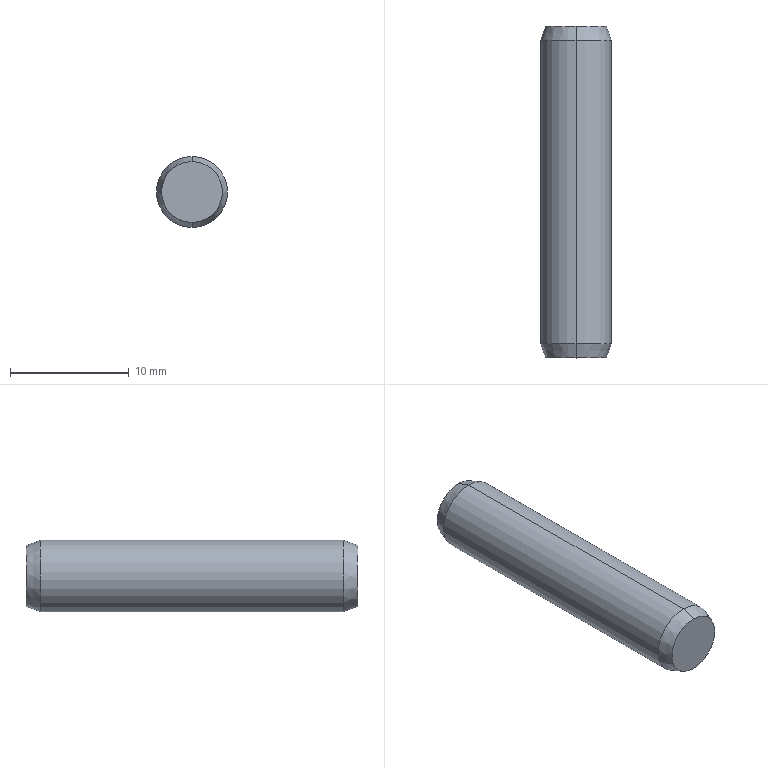Part | SolidWorks | features Chamfer 2, Extrusion 1 | 1 solid | 8 faces | box 6 x 28 x 6 mm | volume 782.281 mm3 | cone 4 | cylinder 2 | plane 2 | commonest cylinder face diameters 6 x2
STEP:
#1=CARTESIAN_POINT('',(0.,-14.,-2.563));
#2=VERTEX_POINT('',#1);
#3=CARTESIAN_POINT('',(0.,-14.,2.563));
#4=VERTEX_POINT('',#3);
#5=CARTESIAN_POINT('',(0.,-14.,0.));
#6=DIRECTION('',(0.,-1.,0.));
#7=DIRECTION('',(0.,0.,1.));
#8=AXIS2_PLACEMENT_3D('',#5,#6,#7);
#9=CIRCLE('',#8,2.563);
#10=EDGE_CURVE('',#2,#4,#9,.T.);
#11=ORIENTED_EDGE('',*,*,#10,.F.);
#12=CARTESIAN_POINT('',(0.,-12.8,-3.));
#13=VERTEX_POINT('',#12);
#14=CARTESIAN_POINT('',(0.,-12.8,-3.));
#15=DIRECTION('',(0.,0.9397,-0.342));
#16=VECTOR('',#15,1000.);
#17=LINE('',#14,#16);
#18=EDGE_CURVE('',#2,#13,#17,.T.);
#19=ORIENTED_EDGE('',*,*,#18,.T.);
#20=CARTESIAN_POINT('',(0.,-12.8,3.));
#21=VERTEX_POINT('',#20);
#22=CARTESIAN_POINT('',(0.,-12.8,0.));
#23=DIRECTION('',(0.,1.,0.));
#24=DIRECTION('',(0.,0.,1.));
#25=AXIS2_PLACEMENT_3D('',#22,#23,#24);
#26=CIRCLE('',#25,3.);
#27=EDGE_CURVE('',#21,#13,#26,.T.);
#28=ORIENTED_EDGE('',*,*,#27,.F.);
#29=CARTESIAN_POINT('',(0.,-12.8,3.));
#30=DIRECTION('',(0.,0.9397,0.342));
#31=VECTOR('',#30,1000.);
#32=LINE('',#29,#31);
#33=EDGE_CURVE('',#4,#21,#32,.T.);
#34=ORIENTED_EDGE('',*,*,#33,.F.);
#35=EDGE_LOOP('',(#11,#19,#28,#34));
#36=FACE_OUTER_BOUND('',#35,.T.);
#37=CARTESIAN_POINT('',(0.,-12.8,0.));
#38=DIRECTION('',(0.,1.,0.));
#39=DIRECTION('',(0.,0.,1.));
#40=AXIS2_PLACEMENT_3D('',#37,#38,#39);
#41=CONICAL_SURFACE('',#40,3.,0.3491);
#42=ADVANCED_FACE('',(#36),#41,.T.);
#43=CARTESIAN_POINT('',(0.,14.,2.563));
#44=VERTEX_POINT('',#43);
#45=CARTESIAN_POINT('',(0.,14.,-2.563));
#46=VERTEX_POINT('',#45);
#47=CARTESIAN_POINT('',(0.,14.,0.));
#48=DIRECTION('',(0.,1.,0.));
#49=DIRECTION('',(0.,0.,1.));
#50=AXIS2_PLACEMENT_3D('',#47,#48,#49);
#51=CIRCLE('',#50,2.563);
#52=EDGE_CURVE('',#44,#46,#51,.T.);
#53=ORIENTED_EDGE('',*,*,#52,.F.);
#54=CARTESIAN_POINT('',(0.,12.8,3.));
#55=VERTEX_POINT('',#54);
#56=CARTESIAN_POINT('',(0.,14.,2.563));
#57=DIRECTION('',(0.,-0.9397,0.342));
#58=VECTOR('',#57,1000.);
#59=LINE('',#56,#58);
#60=EDGE_CURVE('',#44,#55,#59,.T.);
#61=ORIENTED_EDGE('',*,*,#60,.T.);
#62=CARTESIAN_POINT('',(0.,12.8,-3.));
#63=VERTEX_POINT('',#62);
#64=CARTESIAN_POINT('',(0.,12.8,0.));
#65=DIRECTION('',(0.,-1.,0.));
#66=DIRECTION('',(0.,0.,1.));
#67=AXIS2_PLACEMENT_3D('',#64,#65,#66);
#68=CIRCLE('',#67,3.);
#69=EDGE_CURVE('',#63,#55,#68,.T.);
#70=ORIENTED_EDGE('',*,*,#69,.F.);
#71=CARTESIAN_POINT('',(0.,14.,-2.563));
#72=DIRECTION('',(0.,-0.9397,-0.342));
#73=VECTOR('',#72,1000.);
#74=LINE('',#71,#73);
#75=EDGE_CURVE('',#46,#63,#74,.T.);
#76=ORIENTED_EDGE('',*,*,#75,.F.);
#77=EDGE_LOOP('',(#53,#61,#70,#76));
#78=FACE_OUTER_BOUND('',#77,.T.);
#79=CARTESIAN_POINT('',(0.,14.,0.));
#80=DIRECTION('',(0.,-1.,0.));
#81=DIRECTION('',(0.,0.,-1.));
#82=AXIS2_PLACEMENT_3D('',#79,#80,#81);
#83=CONICAL_SURFACE('',#82,2.563,0.3491);
#84=ADVANCED_FACE('',(#78),#83,.T.);
#85=ORIENTED_EDGE('',*,*,#69,.T.);
#86=CARTESIAN_POINT('',(0.,14.,3.));
#87=DIRECTION('',(0.,-1.,0.));
#88=VECTOR('',#87,1000.);
#89=LINE('',#86,#88);
#90=EDGE_CURVE('',#55,#21,#89,.T.);
#91=ORIENTED_EDGE('',*,*,#90,.T.);
#92=ORIENTED_EDGE('',*,*,#27,.T.);
#93=CARTESIAN_POINT('',(0.,14.,-3.));
#94=DIRECTION('',(0.,-1.,0.));
#95=VECTOR('',#94,1000.);
#96=LINE('',#93,#95);
#97=EDGE_CURVE('',#63,#13,#96,.T.);
#98=ORIENTED_EDGE('',*,*,#97,.F.);
#99=EDGE_LOOP('',(#85,#91,#92,#98));
#100=FACE_OUTER_BOUND('',#99,.T.);
#101=CARTESIAN_POINT('',(0.,14.,0.));
#102=DIRECTION('',(0.,-1.,0.));
#103=DIRECTION('',(0.,0.,-1.));
#104=AXIS2_PLACEMENT_3D('',#101,#102,#103);
#105=CYLINDRICAL_SURFACE('',#104,3.);
#106=ADVANCED_FACE('',(#100),#105,.T.);
#107=ORIENTED_EDGE('',*,*,#90,.F.);
#108=CARTESIAN_POINT('',(0.,12.8,0.));
#109=DIRECTION('',(0.,-1.,0.));
#110=DIRECTION('',(0.,0.,1.));
#111=AXIS2_PLACEMENT_3D('',#108,#109,#110);
#112=CIRCLE('',#111,3.);
#113=EDGE_CURVE('',#55,#63,#112,.T.);
#114=ORIENTED_EDGE('',*,*,#113,.T.);
#115=ORIENTED_EDGE('',*,*,#97,.T.);
#116=CARTESIAN_POINT('',(0.,-12.8,0.));
#117=DIRECTION('',(0.,1.,0.));
#118=DIRECTION('',(0.,0.,1.));
#119=AXIS2_PLACEMENT_3D('',#116,#117,#118);
#120=CIRCLE('',#119,3.);
#121=EDGE_CURVE('',#13,#21,#120,.T.);
#122=ORIENTED_EDGE('',*,*,#121,.T.);
#123=EDGE_LOOP('',(#107,#114,#115,#122));
#124=FACE_OUTER_BOUND('',#123,.T.);
#125=CARTESIAN_POINT('',(0.,14.,0.));
#126=DIRECTION('',(0.,-1.,0.));
#127=DIRECTION('',(0.,0.,-1.));
#128=AXIS2_PLACEMENT_3D('',#125,#126,#127);
#129=CYLINDRICAL_SURFACE('',#128,3.);
#130=ADVANCED_FACE('',(#124),#129,.T.);
#131=CARTESIAN_POINT('',(0.,14.,0.));
#132=DIRECTION('',(0.,1.,0.));
#133=DIRECTION('',(0.,0.,1.));
#134=AXIS2_PLACEMENT_3D('',#131,#132,#133);
#135=CIRCLE('',#134,2.563);
#136=EDGE_CURVE('',#46,#44,#135,.T.);
#137=ORIENTED_EDGE('',*,*,#136,.T.);
#138=ORIENTED_EDGE('',*,*,#52,.T.);
#139=EDGE_LOOP('',(#137,#138));
#140=FACE_OUTER_BOUND('',#139,.T.);
#141=CARTESIAN_POINT('',(0.,14.,0.));
#142=DIRECTION('',(0.,1.,0.));
#143=DIRECTION('',(0.,0.,1.));
#144=AXIS2_PLACEMENT_3D('',#141,#142,#143);
#145=PLANE('',#144);
#146=ADVANCED_FACE('',(#140),#145,.T.);
#147=CARTESIAN_POINT('',(0.,-14.,0.));
#148=DIRECTION('',(0.,-1.,0.));
#149=DIRECTION('',(0.,0.,1.));
#150=AXIS2_PLACEMENT_3D('',#147,#148,#149);
#151=CIRCLE('',#150,2.563);
#152=EDGE_CURVE('',#4,#2,#151,.T.);
#153=ORIENTED_EDGE('',*,*,#152,.T.);
#154=ORIENTED_EDGE('',*,*,#10,.T.);
#155=EDGE_LOOP('',(#153,#154));
#156=FACE_OUTER_BOUND('',#155,.T.);
#157=CARTESIAN_POINT('',(0.,-14.,0.));
#158=DIRECTION('',(0.,1.,0.));
#159=DIRECTION('',(0.,0.,1.));
#160=AXIS2_PLACEMENT_3D('',#157,#158,#159);
#161=PLANE('',#160);
#162=ADVANCED_FACE('',(#156),#161,.F.);
#163=ORIENTED_EDGE('',*,*,#60,.F.);
#164=ORIENTED_EDGE('',*,*,#136,.F.);
#165=ORIENTED_EDGE('',*,*,#75,.T.);
#166=ORIENTED_EDGE('',*,*,#113,.F.);
#167=EDGE_LOOP('',(#163,#164,#165,#166));
#168=FACE_OUTER_BOUND('',#167,.T.);
#169=CARTESIAN_POINT('',(0.,14.,0.));
#170=DIRECTION('',(0.,-1.,0.));
#171=DIRECTION('',(0.,0.,-1.));
#172=AXIS2_PLACEMENT_3D('',#169,#170,#171);
#173=CONICAL_SURFACE('',#172,2.563,0.3491);
#174=ADVANCED_FACE('',(#168),#173,.T.);
#175=ORIENTED_EDGE('',*,*,#18,.F.);
#176=ORIENTED_EDGE('',*,*,#152,.F.);
#177=ORIENTED_EDGE('',*,*,#33,.T.);
#178=ORIENTED_EDGE('',*,*,#121,.F.);
#179=EDGE_LOOP('',(#175,#176,#177,#178));
#180=FACE_OUTER_BOUND('',#179,.T.);
#181=CARTESIAN_POINT('',(0.,-12.8,0.));
#182=DIRECTION('',(0.,1.,0.));
#183=DIRECTION('',(0.,0.,1.));
#184=AXIS2_PLACEMENT_3D('',#181,#182,#183);
#185=CONICAL_SURFACE('',#184,3.,0.3491);
#186=ADVANCED_FACE('',(#180),#185,.T.);
#187=CLOSED_SHELL('',(#42,#84,#106,#130,#146,#162,#174,#186));
#188=MANIFOLD_SOLID_BREP('',#187);
#189=CARTESIAN_POINT('',(0.,0.,0.));
#190=DIRECTION('',(0.,0.,1.));
#191=DIRECTION('',(1.,0.,0.));
#192=AXIS2_PLACEMENT_3D('',#189,#190,#191);
#193=(LENGTH_UNIT()NAMED_UNIT(*)SI_UNIT(.MILLI.,.METRE.));
#194=UNCERTAINTY_MEASURE_WITH_UNIT(LENGTH_MEASURE(0.00001),#193,'','');
#195=(NAMED_UNIT(*)PLANE_ANGLE_UNIT()SI_UNIT($,.RADIAN.));
#196=(NAMED_UNIT(*)SI_UNIT($,.STERADIAN.)SOLID_ANGLE_UNIT());
#197=(GEOMETRIC_REPRESENTATION_CONTEXT(3)GLOBAL_UNCERTAINTY_ASSIGNED_CONTEXT((#194))GLOBAL_UNIT_ASSIGNED_CONTEXT((#193,#195,#196))REPRESENTATION_CONTEXT('',''));
#198=ADVANCED_BREP_SHAPE_REPRESENTATION('',(#188,#192),#197);